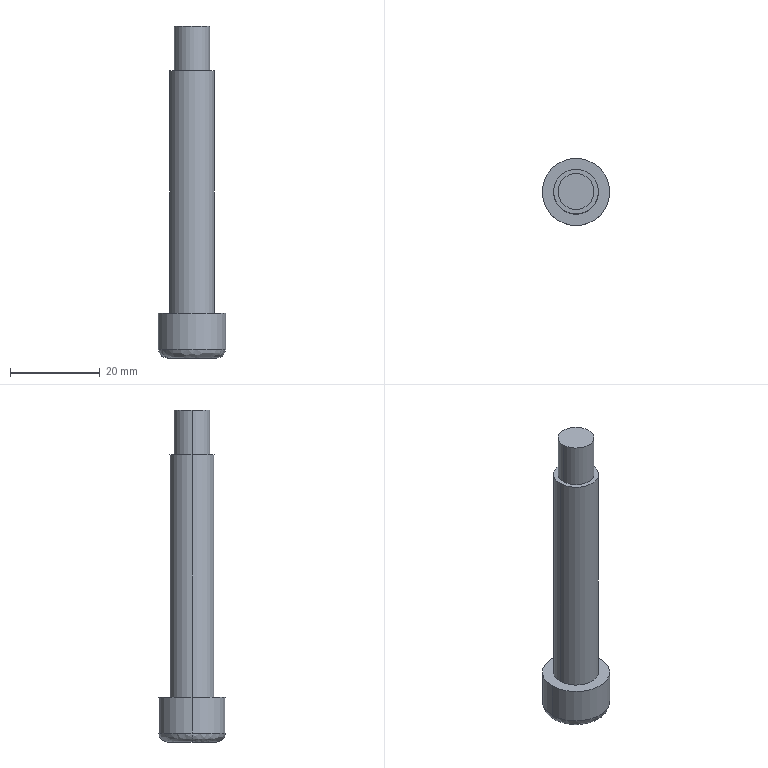Part | STEP file | BULONG BAC M8X10X56 | 1 solid | 19 faces | box 15 x 15 x 74 mm | volume 6196 mm3 | plane 11 | cylinder 6 | spline 2 | commonest cylinder face diameters 8 x2 10 x2 15 x2
STEP:
#1=CARTESIAN_POINT('',(0.,0.,0.));
#2=DIRECTION('',(0.,0.,1.));
#3=DIRECTION('',(1.,0.,0.));
#4=AXIS2_PLACEMENT_3D('',#1,#2,#3);
#5=CARTESIAN_POINT('',(-5.5,0.,0.));
#6=VERTEX_POINT('',#5);
#7=CARTESIAN_POINT('',(5.5,0.,0.));
#8=VERTEX_POINT('',#7);
#9=CARTESIAN_POINT('',(-5.5,0.,0.));
#10=CARTESIAN_POINT('',(-5.5,-11.,0.));
#11=CARTESIAN_POINT('',(5.5,-11.,0.));
#12=CARTESIAN_POINT('',(5.5,0.,0.));
#13=(BOUNDED_CURVE()B_SPLINE_CURVE(3,(#9,#10,#11,#12),.UNSPECIFIED.,.F.,.F.)B_SPLINE_CURVE_WITH_KNOTS((4,4),(0.5,1.),.PIECEWISE_BEZIER_KNOTS.)CURVE()GEOMETRIC_REPRESENTATION_ITEM()RATIONAL_B_SPLINE_CURVE((1.,0.3333,0.3333,1.))REPRESENTATION_ITEM(''));
#14=CARTESIAN_POINT('',(5.5,0.,0.));
#15=CARTESIAN_POINT('',(5.5,-11.,0.));
#16=CARTESIAN_POINT('',(-5.5,-11.,0.));
#17=CARTESIAN_POINT('',(-5.5,0.,0.));
#18=CARTESIAN_POINT('',(6.672,0.,0.));
#19=CARTESIAN_POINT('',(6.672,-13.343,0.));
#20=CARTESIAN_POINT('',(-6.672,-13.343,0.));
#21=CARTESIAN_POINT('',(-6.672,0.,0.));
#22=CARTESIAN_POINT('',(7.5,0.,0.8284));
#23=CARTESIAN_POINT('',(7.5,-15.,0.8284));
#24=CARTESIAN_POINT('',(-7.5,-15.,0.8284));
#25=CARTESIAN_POINT('',(-7.5,0.,0.8284));
#26=CARTESIAN_POINT('',(7.5,0.,2.));
#27=CARTESIAN_POINT('',(7.5,-15.,2.));
#28=CARTESIAN_POINT('',(-7.5,-15.,2.));
#29=CARTESIAN_POINT('',(-7.5,0.,2.));
#30=(BOUNDED_SURFACE()B_SPLINE_SURFACE(3,3,((#14,#15,#16,#17),(#18,#19,#20,#21),(#22,#23,#24,#25),(#26,#27,#28,#29)),.UNSPECIFIED.,.F.,.F.,.F.)B_SPLINE_SURFACE_WITH_KNOTS((4,4),(4,4),(0.,1.),(0.,1.),.PIECEWISE_BEZIER_KNOTS.)GEOMETRIC_REPRESENTATION_ITEM()RATIONAL_B_SPLINE_SURFACE(((1.,0.3333,0.3333,1.),(0.8047,0.2682,0.2682,0.8047),(0.8047,0.2682,0.2682,0.8047),(1.,0.3333,0.3333,1.)))REPRESENTATION_ITEM('')SURFACE());
#31=CARTESIAN_POINT('',(0.,1.));
#32=CARTESIAN_POINT('',(0.,0.));
#33=B_SPLINE_CURVE_WITH_KNOTS('',1,(#31,#32),.UNSPECIFIED.,.F.,.F.,(2,2),(0.5,1.),.PIECEWISE_BEZIER_KNOTS.);
#34=(GEOMETRIC_REPRESENTATION_CONTEXT(2)PARAMETRIC_REPRESENTATION_CONTEXT()REPRESENTATION_CONTEXT('',''));
#35=DEFINITIONAL_REPRESENTATION('',(#33),#34);
#36=PCURVE('',#30,#35);
#37=CARTESIAN_POINT('',(0.,0.,0.));
#38=DIRECTION('',(0.,0.,-1.));
#39=DIRECTION('',(-1.,0.,0.));
#40=AXIS2_PLACEMENT_3D('',#37,#38,#39);
#41=PLANE('',#40);
#42=CARTESIAN_POINT('',(5.5,0.));
#43=CARTESIAN_POINT('',(5.5,-11.));
#44=CARTESIAN_POINT('',(-5.5,-11.));
#45=CARTESIAN_POINT('',(-5.5,0.));
#46=(BOUNDED_CURVE()B_SPLINE_CURVE(3,(#42,#43,#44,#45),.UNSPECIFIED.,.F.,.F.)B_SPLINE_CURVE_WITH_KNOTS((4,4),(0.5,1.),.PIECEWISE_BEZIER_KNOTS.)CURVE()GEOMETRIC_REPRESENTATION_ITEM()RATIONAL_B_SPLINE_CURVE((1.,0.3333,0.3333,1.))REPRESENTATION_ITEM(''));
#47=(GEOMETRIC_REPRESENTATION_CONTEXT(2)PARAMETRIC_REPRESENTATION_CONTEXT()REPRESENTATION_CONTEXT('',''));
#48=DEFINITIONAL_REPRESENTATION('',(#46),#47);
#49=PCURVE('',#41,#48);
#50=SURFACE_CURVE('',#13,(#36,#49),.PCURVE_S1.);
#51=EDGE_CURVE('',#6,#8,#50,.T.);
#52=ORIENTED_EDGE('',*,*,#51,.T.);
#53=CARTESIAN_POINT('',(7.5,0.,2.));
#54=VERTEX_POINT('',#53);
#55=CARTESIAN_POINT('',(5.5,0.,2.));
#56=DIRECTION('',(0.,-1.,0.));
#57=DIRECTION('',(1.,0.,0.));
#58=AXIS2_PLACEMENT_3D('',#55,#56,#57);
#59=CIRCLE('',#58,2.);
#60=CARTESIAN_POINT('',(0.,0.));
#61=CARTESIAN_POINT('',(0.01683,0.));
#62=CARTESIAN_POINT('',(0.04999,0.));
#63=CARTESIAN_POINT('',(0.09843,0.));
#64=CARTESIAN_POINT('',(0.1457,0.));
#65=CARTESIAN_POINT('',(0.192,0.));
#66=CARTESIAN_POINT('',(0.2375,0.));
#67=CARTESIAN_POINT('',(0.2823,0.));
#68=CARTESIAN_POINT('',(0.3265,0.));
#69=CARTESIAN_POINT('',(0.3703,0.));
#70=CARTESIAN_POINT('',(0.4137,0.));
#71=CARTESIAN_POINT('',(0.4569,0.));
#72=CARTESIAN_POINT('',(0.5,0.));
#73=CARTESIAN_POINT('',(0.5431,0.));
#74=CARTESIAN_POINT('',(0.5863,0.));
#75=CARTESIAN_POINT('',(0.6297,0.));
#76=CARTESIAN_POINT('',(0.6735,0.));
#77=CARTESIAN_POINT('',(0.7177,0.));
#78=CARTESIAN_POINT('',(0.7625,0.));
#79=CARTESIAN_POINT('',(0.808,0.));
#80=CARTESIAN_POINT('',(0.8543,0.));
#81=CARTESIAN_POINT('',(0.9016,0.));
#82=CARTESIAN_POINT('',(0.95,0.));
#83=CARTESIAN_POINT('',(0.9832,0.));
#84=CARTESIAN_POINT('',(1.,0.));
#85=B_SPLINE_CURVE_WITH_KNOTS('',3,(#60,#61,#62,#63,#64,#65,#66,#67,#68,#69,#70,#71,#72,#73,#74,#75,#76,#77,#78,#79,#80,#81,#82,#83,#84),.UNSPECIFIED.,.F.,.F.,(4,1,1,1,1,1,1,1,1,1,1,1,1,1,1,1,1,1,1,1,1,1,4),(4.712,4.784,4.855,4.927,4.998,5.069,5.141,5.212,5.284,5.355,5.426,5.498,5.569,5.641,5.712,5.783,5.855,5.926,5.998,6.069,6.14,6.212,6.283),.QUASI_UNIFORM_KNOTS.);
#86=(GEOMETRIC_REPRESENTATION_CONTEXT(2)PARAMETRIC_REPRESENTATION_CONTEXT()REPRESENTATION_CONTEXT('',''));
#87=DEFINITIONAL_REPRESENTATION('',(#85),#86);
#88=PCURVE('',#30,#87);
#89=CARTESIAN_POINT('',(-5.5,0.,0.));
#90=CARTESIAN_POINT('',(-5.5,11.,0.));
#91=CARTESIAN_POINT('',(5.5,11.,0.));
#92=CARTESIAN_POINT('',(5.5,0.,0.));
#93=CARTESIAN_POINT('',(-6.672,0.,0.));
#94=CARTESIAN_POINT('',(-6.672,13.343,0.));
#95=CARTESIAN_POINT('',(6.672,13.343,0.));
#96=CARTESIAN_POINT('',(6.672,0.,0.));
#97=CARTESIAN_POINT('',(-7.5,0.,0.8284));
#98=CARTESIAN_POINT('',(-7.5,15.,0.8284));
#99=CARTESIAN_POINT('',(7.5,15.,0.8284));
#100=CARTESIAN_POINT('',(7.5,0.,0.8284));
#101=CARTESIAN_POINT('',(-7.5,0.,2.));
#102=CARTESIAN_POINT('',(-7.5,15.,2.));
#103=CARTESIAN_POINT('',(7.5,15.,2.));
#104=CARTESIAN_POINT('',(7.5,0.,2.));
#105=(BOUNDED_SURFACE()B_SPLINE_SURFACE(3,3,((#89,#90,#91,#92),(#93,#94,#95,#96),(#97,#98,#99,#100),(#101,#102,#103,#104)),.UNSPECIFIED.,.F.,.F.,.F.)B_SPLINE_SURFACE_WITH_KNOTS((4,4),(4,4),(0.,1.),(0.,1.),.PIECEWISE_BEZIER_KNOTS.)GEOMETRIC_REPRESENTATION_ITEM()RATIONAL_B_SPLINE_SURFACE(((1.,0.3333,0.3333,1.),(0.8047,0.2682,0.2682,0.8047),(0.8047,0.2682,0.2682,0.8047),(1.,0.3333,0.3333,1.)))REPRESENTATION_ITEM('')SURFACE());
#106=CARTESIAN_POINT('',(0.,1.));
#107=CARTESIAN_POINT('',(0.01683,1.));
#108=CARTESIAN_POINT('',(0.04999,1.));
#109=CARTESIAN_POINT('',(0.09843,1.));
#110=CARTESIAN_POINT('',(0.1457,1.));
#111=CARTESIAN_POINT('',(0.192,1.));
#112=CARTESIAN_POINT('',(0.2375,1.));
#113=CARTESIAN_POINT('',(0.2823,1.));
#114=CARTESIAN_POINT('',(0.3265,1.));
#115=CARTESIAN_POINT('',(0.3703,1.));
#116=CARTESIAN_POINT('',(0.4137,1.));
#117=CARTESIAN_POINT('',(0.4569,1.));
#118=CARTESIAN_POINT('',(0.5,1.));
#119=CARTESIAN_POINT('',(0.5431,1.));
#120=CARTESIAN_POINT('',(0.5863,1.));
#121=CARTESIAN_POINT('',(0.6297,1.));
#122=CARTESIAN_POINT('',(0.6735,1.));
#123=CARTESIAN_POINT('',(0.7177,1.));
#124=CARTESIAN_POINT('',(0.7625,1.));
#125=CARTESIAN_POINT('',(0.808,1.));
#126=CARTESIAN_POINT('',(0.8543,1.));
#127=CARTESIAN_POINT('',(0.9016,1.));
#128=CARTESIAN_POINT('',(0.95,1.));
#129=CARTESIAN_POINT('',(0.9832,1.));
#130=CARTESIAN_POINT('',(1.,1.));
#131=B_SPLINE_CURVE_WITH_KNOTS('',3,(#106,#107,#108,#109,#110,#111,#112,#113,#114,#115,#116,#117,#118,#119,#120,#121,#122,#123,#124,#125,#126,#127,#128,#129,#130),.UNSPECIFIED.,.F.,.F.,(4,1,1,1,1,1,1,1,1,1,1,1,1,1,1,1,1,1,1,1,1,1,4),(4.712,4.784,4.855,4.927,4.998,5.069,5.141,5.212,5.284,5.355,5.426,5.498,5.569,5.641,5.712,5.783,5.855,5.926,5.998,6.069,6.14,6.212,6.283),.QUASI_UNIFORM_KNOTS.);
#132=(GEOMETRIC_REPRESENTATION_CONTEXT(2)PARAMETRIC_REPRESENTATION_CONTEXT()REPRESENTATION_CONTEXT('',''));
#133=DEFINITIONAL_REPRESENTATION('',(#131),#132);
#134=PCURVE('',#105,#133);
#135=SURFACE_CURVE('',#59,(#88,#134),.PCURVE_S1.);
#136=EDGE_CURVE('',#8,#54,#135,.T.);
#137=ORIENTED_EDGE('',*,*,#136,.T.);
#138=CARTESIAN_POINT('',(-7.5,0.,2.));
#139=VERTEX_POINT('',#138);
#140=CARTESIAN_POINT('',(0.,0.,2.));
#141=DIRECTION('',(0.,0.,1.));
#142=DIRECTION('',(1.,0.,0.));
#143=AXIS2_PLACEMENT_3D('',#140,#141,#142);
#144=CIRCLE('',#143,7.5);
#145=CARTESIAN_POINT('',(1.,1.));
#146=CARTESIAN_POINT('',(1.,0.9763));
#147=CARTESIAN_POINT('',(1.,0.9319));
#148=CARTESIAN_POINT('',(1.,0.8733));
#149=CARTESIAN_POINT('',(1.,0.8206));
#150=CARTESIAN_POINT('',(1.,0.7724));
#151=CARTESIAN_POINT('',(1.,0.7279));
#152=CARTESIAN_POINT('',(1.,0.6861));
#153=CARTESIAN_POINT('',(1.,0.6465));
#154=CARTESIAN_POINT('',(1.,0.6086));
#155=CARTESIAN_POINT('',(1.,0.5718));
#156=CARTESIAN_POINT('',(1.,0.5357));
#157=CARTESIAN_POINT('',(1.,0.5));
#158=CARTESIAN_POINT('',(1.,0.4643));
#159=CARTESIAN_POINT('',(1.,0.4282));
#160=CARTESIAN_POINT('',(1.,0.3914));
#161=CARTESIAN_POINT('',(1.,0.3535));
#162=CARTESIAN_POINT('',(1.,0.3139));
#163=CARTESIAN_POINT('',(1.,0.2721));
#164=CARTESIAN_POINT('',(1.,0.2276));
#165=CARTESIAN_POINT('',(1.,0.1794));
#166=CARTESIAN_POINT('',(1.,0.1267));
#167=CARTESIAN_POINT('',(1.,0.06805));
#168=CARTESIAN_POINT('',(1.,0.02375));
#169=CARTESIAN_POINT('',(1.,0.));
#170=B_SPLINE_CURVE_WITH_KNOTS('',3,(#145,#146,#147,#148,#149,#150,#151,#152,#153,#154,#155,#156,#157,#158,#159,#160,#161,#162,#163,#164,#165,#166,#167,#168,#169),.UNSPECIFIED.,.F.,.F.,(4,1,1,1,1,1,1,1,1,1,1,1,1,1,1,1,1,1,1,1,1,1,4),(3.142,3.284,3.427,3.57,3.713,3.856,3.998,4.141,4.284,4.427,4.57,4.712,4.855,4.998,5.141,5.284,5.426,5.569,5.712,5.855,5.998,6.14,6.283),.QUASI_UNIFORM_KNOTS.);
#171=(GEOMETRIC_REPRESENTATION_CONTEXT(2)PARAMETRIC_REPRESENTATION_CONTEXT()REPRESENTATION_CONTEXT('',''));
#172=DEFINITIONAL_REPRESENTATION('',(#170),#171);
#173=PCURVE('',#30,#172);
#174=CARTESIAN_POINT('',(0.,0.,0.));
#175=DIRECTION('',(0.,0.,1.));
#176=DIRECTION('',(1.,0.,0.));
#177=AXIS2_PLACEMENT_3D('',#174,#175,#176);
#178=CYLINDRICAL_SURFACE('',#177,7.5);
#179=CARTESIAN_POINT('',(0.,2.));
#180=DIRECTION('',(1.,0.));
#181=VECTOR('',#180,1.);
#182=LINE('',#179,#181);
#183=(GEOMETRIC_REPRESENTATION_CONTEXT(2)PARAMETRIC_REPRESENTATION_CONTEXT()REPRESENTATION_CONTEXT('',''));
#184=DEFINITIONAL_REPRESENTATION('',(#182),#183);
#185=PCURVE('',#178,#184);
#186=SURFACE_CURVE('',#144,(#173,#185),.PCURVE_S1.);
#187=EDGE_CURVE('',#139,#54,#186,.T.);
#188=ORIENTED_EDGE('',*,*,#187,.F.);
#189=CARTESIAN_POINT('',(-5.5,0.,2.));
#190=DIRECTION('',(0.,1.,0.));
#191=DIRECTION('',(-1.,0.,0.));
#192=AXIS2_PLACEMENT_3D('',#189,#190,#191);
#193=CIRCLE('',#192,2.);
#194=CARTESIAN_POINT('',(0.,1.));
#195=CARTESIAN_POINT('',(0.01683,1.));
#196=CARTESIAN_POINT('',(0.04999,1.));
#197=CARTESIAN_POINT('',(0.09843,1.));
#198=CARTESIAN_POINT('',(0.1457,1.));
#199=CARTESIAN_POINT('',(0.192,1.));
#200=CARTESIAN_POINT('',(0.2375,1.));
#201=CARTESIAN_POINT('',(0.2823,1.));
#202=CARTESIAN_POINT('',(0.3265,1.));
#203=CARTESIAN_POINT('',(0.3703,1.));
#204=CARTESIAN_POINT('',(0.4137,1.));
#205=CARTESIAN_POINT('',(0.4569,1.));
#206=CARTESIAN_POINT('',(0.5,1.));
#207=CARTESIAN_POINT('',(0.5431,1.));
#208=CARTESIAN_POINT('',(0.5863,1.));
#209=CARTESIAN_POINT('',(0.6297,1.));
#210=CARTESIAN_POINT('',(0.6735,1.));
#211=CARTESIAN_POINT('',(0.7177,1.));
#212=CARTESIAN_POINT('',(0.7625,1.));
#213=CARTESIAN_POINT('',(0.808,1.));
#214=CARTESIAN_POINT('',(0.8543,1.));
#215=CARTESIAN_POINT('',(0.9016,1.));
#216=CARTESIAN_POINT('',(0.95,1.));
#217=CARTESIAN_POINT('',(0.9832,1.));
#218=CARTESIAN_POINT('',(1.,1.));
#219=B_SPLINE_CURVE_WITH_KNOTS('',3,(#194,#195,#196,#197,#198,#199,#200,#201,#202,#203,#204,#205,#206,#207,#208,#209,#210,#211,#212,#213,#214,#215,#216,#217,#218),.UNSPECIFIED.,.F.,.F.,(4,1,1,1,1,1,1,1,1,1,1,1,1,1,1,1,1,1,1,1,1,1,4),(4.712,4.784,4.855,4.927,4.998,5.069,5.141,5.212,5.284,5.355,5.426,5.498,5.569,5.641,5.712,5.783,5.855,5.926,5.998,6.069,6.14,6.212,6.283),.QUASI_UNIFORM_KNOTS.);
#220=(GEOMETRIC_REPRESENTATION_CONTEXT(2)PARAMETRIC_REPRESENTATION_CONTEXT()REPRESENTATION_CONTEXT('',''));
#221=DEFINITIONAL_REPRESENTATION('',(#219),#220);
#222=PCURVE('',#30,#221);
#223=CARTESIAN_POINT('',(0.,0.));
#224=CARTESIAN_POINT('',(0.01683,0.));
#225=CARTESIAN_POINT('',(0.04999,0.));
#226=CARTESIAN_POINT('',(0.09843,0.));
#227=CARTESIAN_POINT('',(0.1457,0.));
#228=CARTESIAN_POINT('',(0.192,0.));
#229=CARTESIAN_POINT('',(0.2375,0.));
#230=CARTESIAN_POINT('',(0.2823,0.));
#231=CARTESIAN_POINT('',(0.3265,0.));
#232=CARTESIAN_POINT('',(0.3703,0.));
#233=CARTESIAN_POINT('',(0.4137,0.));
#234=CARTESIAN_POINT('',(0.4569,0.));
#235=CARTESIAN_POINT('',(0.5,0.));
#236=CARTESIAN_POINT('',(0.5431,0.));
#237=CARTESIAN_POINT('',(0.5863,0.));
#238=CARTESIAN_POINT('',(0.6297,0.));
#239=CARTESIAN_POINT('',(0.6735,0.));
#240=CARTESIAN_POINT('',(0.7177,0.));
#241=CARTESIAN_POINT('',(0.7625,0.));
#242=CARTESIAN_POINT('',(0.808,0.));
#243=CARTESIAN_POINT('',(0.8543,0.));
#244=CARTESIAN_POINT('',(0.9016,0.));
#245=CARTESIAN_POINT('',(0.95,0.));
#246=CARTESIAN_POINT('',(0.9832,0.));
#247=CARTESIAN_POINT('',(1.,0.));
#248=B_SPLINE_CURVE_WITH_KNOTS('',3,(#223,#224,#225,#226,#227,#228,#229,#230,#231,#232,#233,#234,#235,#236,#237,#238,#239,#240,#241,#242,#243,#244,#245,#246,#247),.UNSPECIFIED.,.F.,.F.,(4,1,1,1,1,1,1,1,1,1,1,1,1,1,1,1,1,1,1,1,1,1,4),(4.712,4.784,4.855,4.927,4.998,5.069,5.141,5.212,5.284,5.355,5.426,5.498,5.569,5.641,5.712,5.783,5.855,5.926,5.998,6.069,6.14,6.212,6.283),.QUASI_UNIFORM_KNOTS.);
#249=(GEOMETRIC_REPRESENTATION_CONTEXT(2)PARAMETRIC_REPRESENTATION_CONTEXT()REPRESENTATION_CONTEXT('',''));
#250=DEFINITIONAL_REPRESENTATION('',(#248),#249);
#251=PCURVE('',#105,#250);
#252=SURFACE_CURVE('',#193,(#222,#251),.PCURVE_S1.);
#253=EDGE_CURVE('',#6,#139,#252,.T.);
#254=ORIENTED_EDGE('',*,*,#253,.F.);
#255=EDGE_LOOP('',(#52,#137,#188,#254));
#256=FACE_BOUND('',#255,.T.);
#257=ADVANCED_FACE('',(#256),#30,.T.);
#258=CARTESIAN_POINT('',(5.,0.,10.));
#259=VERTEX_POINT('',#258);
#260=CARTESIAN_POINT('',(-5.,0.,10.));
#261=VERTEX_POINT('',#260);
#262=CARTESIAN_POINT('',(0.,0.,10.));
#263=DIRECTION('',(0.,0.,1.));
#264=DIRECTION('',(1.,0.,0.));
#265=AXIS2_PLACEMENT_3D('',#262,#263,#264);
#266=CIRCLE('',#265,5.);
#267=CARTESIAN_POINT('',(0.,0.,10.));
#268=DIRECTION('',(0.,0.,1.));
#269=DIRECTION('',(1.,0.,0.));
#270=AXIS2_PLACEMENT_3D('',#267,#268,#269);
#271=CYLINDRICAL_SURFACE('',#270,5.);
#272=CARTESIAN_POINT('',(0.,0.));
#273=DIRECTION('',(1.,0.));
#274=VECTOR('',#273,1.);
#275=LINE('',#272,#274);
#276=(GEOMETRIC_REPRESENTATION_CONTEXT(2)PARAMETRIC_REPRESENTATION_CONTEXT()REPRESENTATION_CONTEXT('',''));
#277=DEFINITIONAL_REPRESENTATION('',(#275),#276);
#278=PCURVE('',#271,#277);
#279=CARTESIAN_POINT('',(0.,0.,10.));
#280=DIRECTION('',(0.,0.,-1.));
#281=DIRECTION('',(-1.,0.,0.));
#282=AXIS2_PLACEMENT_3D('',#279,#280,#281);
#283=PLANE('',#282);
#284=CARTESIAN_POINT('',(-5.,0.));
#285=CARTESIAN_POINT('',(-5.,8.66));
#286=CARTESIAN_POINT('',(2.5,4.33));
#287=CARTESIAN_POINT('',(10.,0.));
#288=CARTESIAN_POINT('',(2.5,-4.33));
#289=CARTESIAN_POINT('',(-5.,-8.66));
#290=CARTESIAN_POINT('',(-5.,0.));
#291=(BOUNDED_CURVE()B_SPLINE_CURVE(2,(#284,#285,#286,#287,#288,#289,#290),.UNSPECIFIED.,.T.,.F.)B_SPLINE_CURVE_WITH_KNOTS((1,2,2,2,2,1),(-2.094,0.,2.094,4.189,6.283,8.378),.UNSPECIFIED.)CURVE()GEOMETRIC_REPRESENTATION_ITEM()RATIONAL_B_SPLINE_CURVE((1.,0.5,1.,0.5,1.,0.5,1.))REPRESENTATION_ITEM(''));
#292=(GEOMETRIC_REPRESENTATION_CONTEXT(2)PARAMETRIC_REPRESENTATION_CONTEXT()REPRESENTATION_CONTEXT('',''));
#293=DEFINITIONAL_REPRESENTATION('',(#291),#292);
#294=PCURVE('',#283,#293);
#295=SURFACE_CURVE('',#266,(#278,#294),.PCURVE_S1.);
#296=EDGE_CURVE('',#259,#261,#295,.T.);
#297=ORIENTED_EDGE('',*,*,#296,.T.);
#298=CARTESIAN_POINT('',(-5.,0.,64.));
#299=VERTEX_POINT('',#298);
#300=CARTESIAN_POINT('',(-5.,0.,10.));
#301=DIRECTION('',(0.,0.,1.));
#302=VECTOR('',#301,1.);
#303=LINE('',#300,#302);
#304=CARTESIAN_POINT('',(3.142,0.));
#305=DIRECTION('',(0.,1.));
#306=VECTOR('',#305,1.);
#307=LINE('',#304,#306);
#308=(GEOMETRIC_REPRESENTATION_CONTEXT(2)PARAMETRIC_REPRESENTATION_CONTEXT()REPRESENTATION_CONTEXT('',''));
#309=DEFINITIONAL_REPRESENTATION('',(#307),#308);
#310=PCURVE('',#271,#309);
#311=CARTESIAN_POINT('',(0.,0.,10.));
#312=DIRECTION('',(0.,0.,1.));
#313=DIRECTION('',(1.,0.,0.));
#314=AXIS2_PLACEMENT_3D('',#311,#312,#313);
#315=CYLINDRICAL_SURFACE('',#314,5.);
#316=CARTESIAN_POINT('',(3.142,0.));
#317=DIRECTION('',(0.,1.));
#318=VECTOR('',#317,1.);
#319=LINE('',#316,#318);
#320=(GEOMETRIC_REPRESENTATION_CONTEXT(2)PARAMETRIC_REPRESENTATION_CONTEXT()REPRESENTATION_CONTEXT('',''));
#321=DEFINITIONAL_REPRESENTATION('',(#319),#320);
#322=PCURVE('',#315,#321);
#323=SURFACE_CURVE('',#303,(#310,#322),.PCURVE_S1.);
#324=EDGE_CURVE('',#261,#299,#323,.T.);
#325=ORIENTED_EDGE('',*,*,#324,.T.);
#326=CARTESIAN_POINT('',(5.,0.,64.));
#327=VERTEX_POINT('',#326);
#328=CARTESIAN_POINT('',(0.,0.,64.));
#329=DIRECTION('',(0.,0.,-1.));
#330=DIRECTION('',(1.,0.,0.));
#331=AXIS2_PLACEMENT_3D('',#328,#329,#330);
#332=CIRCLE('',#331,5.);
#333=CARTESIAN_POINT('',(6.283,54.));
#334=DIRECTION('',(-1.,0.));
#335=VECTOR('',#334,1.);
#336=LINE('',#333,#335);
#337=(GEOMETRIC_REPRESENTATION_CONTEXT(2)PARAMETRIC_REPRESENTATION_CONTEXT()REPRESENTATION_CONTEXT('',''));
#338=DEFINITIONAL_REPRESENTATION('',(#336),#337);
#339=PCURVE('',#271,#338);
#340=CARTESIAN_POINT('',(0.,0.,64.));
#341=DIRECTION('',(0.,0.,-1.));
#342=DIRECTION('',(-1.,0.,0.));
#343=AXIS2_PLACEMENT_3D('',#340,#341,#342);
#344=PLANE('',#343);
#345=CARTESIAN_POINT('',(0.,0.));
#346=DIRECTION('',(-1.,0.));
#347=AXIS2_PLACEMENT_2D('',#345,#346);
#348=CIRCLE('',#347,5.);
#349=(GEOMETRIC_REPRESENTATION_CONTEXT(2)PARAMETRIC_REPRESENTATION_CONTEXT()REPRESENTATION_CONTEXT('',''));
#350=DEFINITIONAL_REPRESENTATION('',(#348),#349);
#351=PCURVE('',#344,#350);
#352=SURFACE_CURVE('',#332,(#339,#351),.PCURVE_S1.);
#353=EDGE_CURVE('',#299,#327,#352,.T.);
#354=ORIENTED_EDGE('',*,*,#353,.T.);
#355=CARTESIAN_POINT('',(5.,0.,10.));
#356=DIRECTION('',(0.,0.,1.));
#357=VECTOR('',#356,1.);
#358=LINE('',#355,#357);
#359=CARTESIAN_POINT('',(0.,0.));
#360=DIRECTION('',(0.,1.));
#361=VECTOR('',#360,1.);
#362=LINE('',#359,#361);
#363=(GEOMETRIC_REPRESENTATION_CONTEXT(2)PARAMETRIC_REPRESENTATION_CONTEXT()REPRESENTATION_CONTEXT('',''));
#364=DEFINITIONAL_REPRESENTATION('',(#362),#363);
#365=PCURVE('',#271,#364);
#366=CARTESIAN_POINT('',(6.283,0.));
#367=DIRECTION('',(0.,1.));
#368=VECTOR('',#367,1.);
#369=LINE('',#366,#368);
#370=(GEOMETRIC_REPRESENTATION_CONTEXT(2)PARAMETRIC_REPRESENTATION_CONTEXT()REPRESENTATION_CONTEXT('',''));
#371=DEFINITIONAL_REPRESENTATION('',(#369),#370);
#372=PCURVE('',#315,#371);
#373=SURFACE_CURVE('',#358,(#365,#372),.PCURVE_S1.);
#374=EDGE_CURVE('',#259,#327,#373,.T.);
#375=ORIENTED_EDGE('',*,*,#374,.F.);
#376=EDGE_LOOP('',(#297,#325,#354,#375));
#377=FACE_BOUND('',#376,.T.);
#378=ADVANCED_FACE('',(#377),#271,.T.);
#379=CARTESIAN_POINT('',(0.,0.,2.));
#380=DIRECTION('',(0.,0.,1.));
#381=DIRECTION('',(1.,0.,0.));
#382=AXIS2_PLACEMENT_3D('',#379,#380,#381);
#383=CIRCLE('',#382,7.5);
#384=CARTESIAN_POINT('',(0.,0.,0.));
#385=DIRECTION('',(0.,0.,1.));
#386=DIRECTION('',(1.,0.,0.));
#387=AXIS2_PLACEMENT_3D('',#384,#385,#386);
#388=CYLINDRICAL_SURFACE('',#387,7.5);
#389=CARTESIAN_POINT('',(0.,2.));
#390=DIRECTION('',(1.,0.));
#391=VECTOR('',#390,1.);
#392=LINE('',#389,#391);
#393=(GEOMETRIC_REPRESENTATION_CONTEXT(2)PARAMETRIC_REPRESENTATION_CONTEXT()REPRESENTATION_CONTEXT('',''));
#394=DEFINITIONAL_REPRESENTATION('',(#392),#393);
#395=PCURVE('',#388,#394);
#396=CARTESIAN_POINT('',(1.,1.));
#397=CARTESIAN_POINT('',(1.,0.9763));
#398=CARTESIAN_POINT('',(1.,0.9319));
#399=CARTESIAN_POINT('',(1.,0.8733));
#400=CARTESIAN_POINT('',(1.,0.8206));
#401=CARTESIAN_POINT('',(1.,0.7724));
#402=CARTESIAN_POINT('',(1.,0.7279));
#403=CARTESIAN_POINT('',(1.,0.6861));
#404=CARTESIAN_POINT('',(1.,0.6465));
#405=CARTESIAN_POINT('',(1.,0.6086));
#406=CARTESIAN_POINT('',(1.,0.5718));
#407=CARTESIAN_POINT('',(1.,0.5357));
#408=CARTESIAN_POINT('',(1.,0.5));
#409=CARTESIAN_POINT('',(1.,0.4643));
#410=CARTESIAN_POINT('',(1.,0.4282));
#411=CARTESIAN_POINT('',(1.,0.3914));
#412=CARTESIAN_POINT('',(1.,0.3535));
#413=CARTESIAN_POINT('',(1.,0.3139));
#414=CARTESIAN_POINT('',(1.,0.2721));
#415=CARTESIAN_POINT('',(1.,0.2276));
#416=CARTESIAN_POINT('',(1.,0.1794));
#417=CARTESIAN_POINT('',(1.,0.1267));
#418=CARTESIAN_POINT('',(1.,0.06805));
#419=CARTESIAN_POINT('',(1.,0.02375));
#420=CARTESIAN_POINT('',(1.,0.));
#421=B_SPLINE_CURVE_WITH_KNOTS('',3,(#396,#397,#398,#399,#400,#401,#402,#403,#404,#405,#406,#407,#408,#409,#410,#411,#412,#413,#414,#415,#416,#417,#418,#419,#420),.UNSPECIFIED.,.F.,.F.,(4,1,1,1,1,1,1,1,1,1,1,1,1,1,1,1,1,1,1,1,1,1,4),(0.,0.1428,0.2856,0.4284,0.5712,0.714,0.8568,0.9996,1.142,1.285,1.428,1.571,1.714,1.856,1.999,2.142,2.285,2.428,2.57,2.713,2.856,2.999,3.142),.QUASI_UNIFORM_KNOTS.);
#422=(GEOMETRIC_REPRESENTATION_CONTEXT(2)PARAMETRIC_REPRESENTATION_CONTEXT()REPRESENTATION_CONTEXT('',''));
#423=DEFINITIONAL_REPRESENTATION('',(#421),#422);
#424=PCURVE('',#105,#423);
#425=SURFACE_CURVE('',#383,(#395,#424),.PCURVE_S1.);
#426=EDGE_CURVE('',#54,#139,#425,.T.);
#427=ORIENTED_EDGE('',*,*,#426,.T.);
#428=CARTESIAN_POINT('',(-7.5,0.,10.));
#429=VERTEX_POINT('',#428);
#430=CARTESIAN_POINT('',(-7.5,0.,0.));
#431=DIRECTION('',(0.,0.,1.));
#432=VECTOR('',#431,1.);
#433=LINE('',#430,#432);
#434=CARTESIAN_POINT('',(3.142,0.));
#435=DIRECTION('',(0.,1.));
#436=VECTOR('',#435,1.);
#437=LINE('',#434,#436);
#438=(GEOMETRIC_REPRESENTATION_CONTEXT(2)PARAMETRIC_REPRESENTATION_CONTEXT()REPRESENTATION_CONTEXT('',''));
#439=DEFINITIONAL_REPRESENTATION('',(#437),#438);
#440=PCURVE('',#388,#439);
#441=CARTESIAN_POINT('',(3.142,0.));
#442=DIRECTION('',(0.,1.));
#443=VECTOR('',#442,1.);
#444=LINE('',#441,#443);
#445=(GEOMETRIC_REPRESENTATION_CONTEXT(2)PARAMETRIC_REPRESENTATION_CONTEXT()REPRESENTATION_CONTEXT('',''));
#446=DEFINITIONAL_REPRESENTATION('',(#444),#445);
#447=PCURVE('',#178,#446);
#448=SURFACE_CURVE('',#433,(#440,#447),.PCURVE_S1.);
#449=EDGE_CURVE('',#139,#429,#448,.T.);
#450=ORIENTED_EDGE('',*,*,#449,.T.);
#451=CARTESIAN_POINT('',(7.5,0.,10.));
#452=VERTEX_POINT('',#451);
#453=CARTESIAN_POINT('',(0.,0.,10.));
#454=DIRECTION('',(0.,0.,-1.));
#455=DIRECTION('',(1.,0.,0.));
#456=AXIS2_PLACEMENT_3D('',#453,#454,#455);
#457=CIRCLE('',#456,7.5);
#458=CARTESIAN_POINT('',(6.283,10.));
#459=DIRECTION('',(-1.,0.));
#460=VECTOR('',#459,1.);
#461=LINE('',#458,#460);
#462=(GEOMETRIC_REPRESENTATION_CONTEXT(2)PARAMETRIC_REPRESENTATION_CONTEXT()REPRESENTATION_CONTEXT('',''));
#463=DEFINITIONAL_REPRESENTATION('',(#461),#462);
#464=PCURVE('',#388,#463);
#465=CARTESIAN_POINT('',(0.,0.));
#466=DIRECTION('',(-1.,0.));
#467=AXIS2_PLACEMENT_2D('',#465,#466);
#468=CIRCLE('',#467,7.5);
#469=(GEOMETRIC_REPRESENTATION_CONTEXT(2)PARAMETRIC_REPRESENTATION_CONTEXT()REPRESENTATION_CONTEXT('',''));
#470=DEFINITIONAL_REPRESENTATION('',(#468),#469);
#471=PCURVE('',#283,#470);
#472=SURFACE_CURVE('',#457,(#464,#471),.PCURVE_S1.);
#473=EDGE_CURVE('',#429,#452,#472,.T.);
#474=ORIENTED_EDGE('',*,*,#473,.T.);
#475=CARTESIAN_POINT('',(7.5,0.,0.));
#476=DIRECTION('',(0.,0.,1.));
#477=VECTOR('',#476,1.);
#478=LINE('',#475,#477);
#479=CARTESIAN_POINT('',(0.,0.));
#480=DIRECTION('',(0.,1.));
#481=VECTOR('',#480,1.);
#482=LINE('',#479,#481);
#483=(GEOMETRIC_REPRESENTATION_CONTEXT(2)PARAMETRIC_REPRESENTATION_CONTEXT()REPRESENTATION_CONTEXT('',''));
#484=DEFINITIONAL_REPRESENTATION('',(#482),#483);
#485=PCURVE('',#388,#484);
#486=CARTESIAN_POINT('',(6.283,0.));
#487=DIRECTION('',(0.,1.));
#488=VECTOR('',#487,1.);
#489=LINE('',#486,#488);
#490=(GEOMETRIC_REPRESENTATION_CONTEXT(2)PARAMETRIC_REPRESENTATION_CONTEXT()REPRESENTATION_CONTEXT('',''));
#491=DEFINITIONAL_REPRESENTATION('',(#489),#490);
#492=PCURVE('',#178,#491);
#493=SURFACE_CURVE('',#478,(#485,#492),.PCURVE_S1.);
#494=EDGE_CURVE('',#54,#452,#493,.T.);
#495=ORIENTED_EDGE('',*,*,#494,.F.);
#496=EDGE_LOOP('',(#427,#450,#474,#495));
#497=FACE_BOUND('',#496,.T.);
#498=ADVANCED_FACE('',(#497),#388,.T.);
#499=CARTESIAN_POINT('',(4.,0.,64.));
#500=VERTEX_POINT('',#499);
#501=CARTESIAN_POINT('',(-4.,0.,64.));
#502=VERTEX_POINT('',#501);
#503=CARTESIAN_POINT('',(0.,0.,64.));
#504=DIRECTION('',(0.,0.,1.));
#505=DIRECTION('',(1.,0.,0.));
#506=AXIS2_PLACEMENT_3D('',#503,#504,#505);
#507=CIRCLE('',#506,4.);
#508=CARTESIAN_POINT('',(0.,0.,64.));
#509=DIRECTION('',(0.,0.,1.));
#510=DIRECTION('',(1.,0.,0.));
#511=AXIS2_PLACEMENT_3D('',#508,#509,#510);
#512=CYLINDRICAL_SURFACE('',#511,4.);
#513=CARTESIAN_POINT('',(0.,0.));
#514=DIRECTION('',(1.,0.));
#515=VECTOR('',#514,1.);
#516=LINE('',#513,#515);
#517=(GEOMETRIC_REPRESENTATION_CONTEXT(2)PARAMETRIC_REPRESENTATION_CONTEXT()REPRESENTATION_CONTEXT('',''));
#518=DEFINITIONAL_REPRESENTATION('',(#516),#517);
#519=PCURVE('',#512,#518);
#520=CARTESIAN_POINT('',(-4.,0.));
#521=CARTESIAN_POINT('',(-4.,6.928));
#522=CARTESIAN_POINT('',(2.,3.464));
#523=CARTESIAN_POINT('',(8.,0.));
#524=CARTESIAN_POINT('',(2.,-3.464));
#525=CARTESIAN_POINT('',(-4.,-6.928));
#526=CARTESIAN_POINT('',(-4.,0.));
#527=(BOUNDED_CURVE()B_SPLINE_CURVE(2,(#520,#521,#522,#523,#524,#525,#526),.UNSPECIFIED.,.T.,.F.)B_SPLINE_CURVE_WITH_KNOTS((1,2,2,2,2,1),(-2.094,0.,2.094,4.189,6.283,8.378),.UNSPECIFIED.)CURVE()GEOMETRIC_REPRESENTATION_ITEM()RATIONAL_B_SPLINE_CURVE((1.,0.5,1.,0.5,1.,0.5,1.))REPRESENTATION_ITEM(''));
#528=(GEOMETRIC_REPRESENTATION_CONTEXT(2)PARAMETRIC_REPRESENTATION_CONTEXT()REPRESENTATION_CONTEXT('',''));
#529=DEFINITIONAL_REPRESENTATION('',(#527),#528);
#530=PCURVE('',#344,#529);
#531=SURFACE_CURVE('',#507,(#519,#530),.PCURVE_S1.);
#532=EDGE_CURVE('',#500,#502,#531,.T.);
#533=ORIENTED_EDGE('',*,*,#532,.T.);
#534=CARTESIAN_POINT('',(-4.,0.,74.));
#535=VERTEX_POINT('',#534);
#536=CARTESIAN_POINT('',(-4.,0.,64.));
#537=DIRECTION('',(0.,0.,1.));
#538=VECTOR('',#537,1.);
#539=LINE('',#536,#538);
#540=CARTESIAN_POINT('',(3.142,0.));
#541=DIRECTION('',(0.,1.));
#542=VECTOR('',#541,1.);
#543=LINE('',#540,#542);
#544=(GEOMETRIC_REPRESENTATION_CONTEXT(2)PARAMETRIC_REPRESENTATION_CONTEXT()REPRESENTATION_CONTEXT('',''));
#545=DEFINITIONAL_REPRESENTATION('',(#543),#544);
#546=PCURVE('',#512,#545);
#547=CARTESIAN_POINT('',(0.,0.,64.));
#548=DIRECTION('',(0.,0.,1.));
#549=DIRECTION('',(1.,0.,0.));
#550=AXIS2_PLACEMENT_3D('',#547,#548,#549);
#551=CYLINDRICAL_SURFACE('',#550,4.);
#552=CARTESIAN_POINT('',(3.142,0.));
#553=DIRECTION('',(0.,1.));
#554=VECTOR('',#553,1.);
#555=LINE('',#552,#554);
#556=(GEOMETRIC_REPRESENTATION_CONTEXT(2)PARAMETRIC_REPRESENTATION_CONTEXT()REPRESENTATION_CONTEXT('',''));
#557=DEFINITIONAL_REPRESENTATION('',(#555),#556);
#558=PCURVE('',#551,#557);
#559=SURFACE_CURVE('',#539,(#546,#558),.PCURVE_S1.);
#560=EDGE_CURVE('',#502,#535,#559,.T.);
#561=ORIENTED_EDGE('',*,*,#560,.T.);
#562=CARTESIAN_POINT('',(4.,0.,74.));
#563=VERTEX_POINT('',#562);
#564=CARTESIAN_POINT('',(0.,0.,74.));
#565=DIRECTION('',(0.,0.,-1.));
#566=DIRECTION('',(1.,0.,0.));
#567=AXIS2_PLACEMENT_3D('',#564,#565,#566);
#568=CIRCLE('',#567,4.);
#569=CARTESIAN_POINT('',(6.283,10.));
#570=DIRECTION('',(-1.,0.));
#571=VECTOR('',#570,1.);
#572=LINE('',#569,#571);
#573=(GEOMETRIC_REPRESENTATION_CONTEXT(2)PARAMETRIC_REPRESENTATION_CONTEXT()REPRESENTATION_CONTEXT('',''));
#574=DEFINITIONAL_REPRESENTATION('',(#572),#573);
#575=PCURVE('',#512,#574);
#576=CARTESIAN_POINT('',(0.,0.,74.));
#577=DIRECTION('',(0.,0.,-1.));
#578=DIRECTION('',(-1.,0.,0.));
#579=AXIS2_PLACEMENT_3D('',#576,#577,#578);
#580=PLANE('',#579);
#581=CARTESIAN_POINT('',(0.,0.));
#582=DIRECTION('',(-1.,0.));
#583=AXIS2_PLACEMENT_2D('',#581,#582);
#584=CIRCLE('',#583,4.);
#585=(GEOMETRIC_REPRESENTATION_CONTEXT(2)PARAMETRIC_REPRESENTATION_CONTEXT()REPRESENTATION_CONTEXT('',''));
#586=DEFINITIONAL_REPRESENTATION('',(#584),#585);
#587=PCURVE('',#580,#586);
#588=SURFACE_CURVE('',#568,(#575,#587),.PCURVE_S1.);
#589=EDGE_CURVE('',#535,#563,#588,.T.);
#590=ORIENTED_EDGE('',*,*,#589,.T.);
#591=CARTESIAN_POINT('',(4.,0.,64.));
#592=DIRECTION('',(0.,0.,1.));
#593=VECTOR('',#592,1.);
#594=LINE('',#591,#593);
#595=CARTESIAN_POINT('',(0.,0.));
#596=DIRECTION('',(0.,1.));
#597=VECTOR('',#596,1.);
#598=LINE('',#595,#597);
#599=(GEOMETRIC_REPRESENTATION_CONTEXT(2)PARAMETRIC_REPRESENTATION_CONTEXT()REPRESENTATION_CONTEXT('',''));
#600=DEFINITIONAL_REPRESENTATION('',(#598),#599);
#601=PCURVE('',#512,#600);
#602=CARTESIAN_POINT('',(6.283,0.));
#603=DIRECTION('',(0.,1.));
#604=VECTOR('',#603,1.);
#605=LINE('',#602,#604);
#606=(GEOMETRIC_REPRESENTATION_CONTEXT(2)PARAMETRIC_REPRESENTATION_CONTEXT()REPRESENTATION_CONTEXT('',''));
#607=DEFINITIONAL_REPRESENTATION('',(#605),#606);
#608=PCURVE('',#551,#607);
#609=SURFACE_CURVE('',#594,(#601,#608),.PCURVE_S1.);
#610=EDGE_CURVE('',#500,#563,#609,.T.);
#611=ORIENTED_EDGE('',*,*,#610,.F.);
#612=EDGE_LOOP('',(#533,#561,#590,#611));
#613=FACE_BOUND('',#612,.T.);
#614=ADVANCED_FACE('',(#613),#512,.T.);
#615=ORIENTED_EDGE('',*,*,#324,.F.);
#616=CARTESIAN_POINT('',(0.,0.,10.));
#617=DIRECTION('',(0.,0.,1.));
#618=DIRECTION('',(1.,0.,0.));
#619=AXIS2_PLACEMENT_3D('',#616,#617,#618);
#620=CIRCLE('',#619,5.);
#621=CARTESIAN_POINT('',(0.,0.));
#622=DIRECTION('',(1.,0.));
#623=VECTOR('',#622,1.);
#624=LINE('',#621,#623);
#625=(GEOMETRIC_REPRESENTATION_CONTEXT(2)PARAMETRIC_REPRESENTATION_CONTEXT()REPRESENTATION_CONTEXT('',''));
#626=DEFINITIONAL_REPRESENTATION('',(#624),#625);
#627=PCURVE('',#315,#626);
#628=CARTESIAN_POINT('',(-5.,0.));
#629=CARTESIAN_POINT('',(-5.,8.66));
#630=CARTESIAN_POINT('',(2.5,4.33));
#631=CARTESIAN_POINT('',(10.,0.));
#632=CARTESIAN_POINT('',(2.5,-4.33));
#633=CARTESIAN_POINT('',(-5.,-8.66));
#634=CARTESIAN_POINT('',(-5.,0.));
#635=(BOUNDED_CURVE()B_SPLINE_CURVE(2,(#628,#629,#630,#631,#632,#633,#634),.UNSPECIFIED.,.T.,.F.)B_SPLINE_CURVE_WITH_KNOTS((1,2,2,2,2,1),(-2.094,0.,2.094,4.189,6.283,8.378),.UNSPECIFIED.)CURVE()GEOMETRIC_REPRESENTATION_ITEM()RATIONAL_B_SPLINE_CURVE((1.,0.5,1.,0.5,1.,0.5,1.))REPRESENTATION_ITEM(''));
#636=(GEOMETRIC_REPRESENTATION_CONTEXT(2)PARAMETRIC_REPRESENTATION_CONTEXT()REPRESENTATION_CONTEXT('',''));
#637=DEFINITIONAL_REPRESENTATION('',(#635),#636);
#638=PCURVE('',#283,#637);
#639=SURFACE_CURVE('',#620,(#627,#638),.PCURVE_S1.);
#640=EDGE_CURVE('',#261,#259,#639,.T.);
#641=ORIENTED_EDGE('',*,*,#640,.T.);
#642=ORIENTED_EDGE('',*,*,#374,.T.);
#643=CARTESIAN_POINT('',(0.,0.,64.));
#644=DIRECTION('',(0.,0.,-1.));
#645=DIRECTION('',(1.,0.,0.));
#646=AXIS2_PLACEMENT_3D('',#643,#644,#645);
#647=CIRCLE('',#646,5.);
#648=CARTESIAN_POINT('',(6.283,54.));
#649=DIRECTION('',(-1.,0.));
#650=VECTOR('',#649,1.);
#651=LINE('',#648,#650);
#652=(GEOMETRIC_REPRESENTATION_CONTEXT(2)PARAMETRIC_REPRESENTATION_CONTEXT()REPRESENTATION_CONTEXT('',''));
#653=DEFINITIONAL_REPRESENTATION('',(#651),#652);
#654=PCURVE('',#315,#653);
#655=CARTESIAN_POINT('',(0.,0.));
#656=DIRECTION('',(-1.,0.));
#657=AXIS2_PLACEMENT_2D('',#655,#656);
#658=CIRCLE('',#657,5.);
#659=(GEOMETRIC_REPRESENTATION_CONTEXT(2)PARAMETRIC_REPRESENTATION_CONTEXT()REPRESENTATION_CONTEXT('',''));
#660=DEFINITIONAL_REPRESENTATION('',(#658),#659);
#661=PCURVE('',#344,#660);
#662=SURFACE_CURVE('',#647,(#654,#661),.PCURVE_S1.);
#663=EDGE_CURVE('',#327,#299,#662,.T.);
#664=ORIENTED_EDGE('',*,*,#663,.T.);
#665=EDGE_LOOP('',(#615,#641,#642,#664));
#666=FACE_BOUND('',#665,.T.);
#667=ADVANCED_FACE('',(#666),#315,.T.);
#668=ORIENTED_EDGE('',*,*,#296,.F.);
#669=ORIENTED_EDGE('',*,*,#640,.F.);
#670=EDGE_LOOP('',(#668,#669));
#671=FACE_BOUND('',#670,.T.);
#672=CARTESIAN_POINT('',(0.,0.,10.));
#673=DIRECTION('',(0.,0.,-1.));
#674=DIRECTION('',(1.,0.,0.));
#675=AXIS2_PLACEMENT_3D('',#672,#673,#674);
#676=CIRCLE('',#675,7.5);
#677=CARTESIAN_POINT('',(0.,0.));
#678=DIRECTION('',(-1.,0.));
#679=AXIS2_PLACEMENT_2D('',#677,#678);
#680=CIRCLE('',#679,7.5);
#681=(GEOMETRIC_REPRESENTATION_CONTEXT(2)PARAMETRIC_REPRESENTATION_CONTEXT()REPRESENTATION_CONTEXT('',''));
#682=DEFINITIONAL_REPRESENTATION('',(#680),#681);
#683=PCURVE('',#283,#682);
#684=CARTESIAN_POINT('',(6.283,10.));
#685=DIRECTION('',(-1.,0.));
#686=VECTOR('',#685,1.);
#687=LINE('',#684,#686);
#688=(GEOMETRIC_REPRESENTATION_CONTEXT(2)PARAMETRIC_REPRESENTATION_CONTEXT()REPRESENTATION_CONTEXT('',''));
#689=DEFINITIONAL_REPRESENTATION('',(#687),#688);
#690=PCURVE('',#178,#689);
#691=SURFACE_CURVE('',#676,(#683,#690),.PCURVE_S1.);
#692=EDGE_CURVE('',#452,#429,#691,.T.);
#693=ORIENTED_EDGE('',*,*,#692,.F.);
#694=ORIENTED_EDGE('',*,*,#473,.F.);
#695=EDGE_LOOP('',(#693,#694));
#696=FACE_BOUND('',#695,.T.);
#697=ADVANCED_FACE('',(#671,#696),#283,.F.);
#698=ORIENTED_EDGE('',*,*,#532,.F.);
#699=CARTESIAN_POINT('',(0.,0.,64.));
#700=DIRECTION('',(0.,0.,1.));
#701=DIRECTION('',(1.,0.,0.));
#702=AXIS2_PLACEMENT_3D('',#699,#700,#701);
#703=CIRCLE('',#702,4.);
#704=CARTESIAN_POINT('',(-4.,0.));
#705=CARTESIAN_POINT('',(-4.,6.928));
#706=CARTESIAN_POINT('',(2.,3.464));
#707=CARTESIAN_POINT('',(8.,0.));
#708=CARTESIAN_POINT('',(2.,-3.464));
#709=CARTESIAN_POINT('',(-4.,-6.928));
#710=CARTESIAN_POINT('',(-4.,0.));
#711=(BOUNDED_CURVE()B_SPLINE_CURVE(2,(#704,#705,#706,#707,#708,#709,#710),.UNSPECIFIED.,.T.,.F.)B_SPLINE_CURVE_WITH_KNOTS((1,2,2,2,2,1),(-2.094,0.,2.094,4.189,6.283,8.378),.UNSPECIFIED.)CURVE()GEOMETRIC_REPRESENTATION_ITEM()RATIONAL_B_SPLINE_CURVE((1.,0.5,1.,0.5,1.,0.5,1.))REPRESENTATION_ITEM(''));
#712=(GEOMETRIC_REPRESENTATION_CONTEXT(2)PARAMETRIC_REPRESENTATION_CONTEXT()REPRESENTATION_CONTEXT('',''));
#713=DEFINITIONAL_REPRESENTATION('',(#711),#712);
#714=PCURVE('',#344,#713);
#715=CARTESIAN_POINT('',(0.,0.));
#716=DIRECTION('',(1.,0.));
#717=VECTOR('',#716,1.);
#718=LINE('',#715,#717);
#719=(GEOMETRIC_REPRESENTATION_CONTEXT(2)PARAMETRIC_REPRESENTATION_CONTEXT()REPRESENTATION_CONTEXT('',''));
#720=DEFINITIONAL_REPRESENTATION('',(#718),#719);
#721=PCURVE('',#551,#720);
#722=SURFACE_CURVE('',#703,(#714,#721),.PCURVE_S1.);
#723=EDGE_CURVE('',#502,#500,#722,.T.);
#724=ORIENTED_EDGE('',*,*,#723,.F.);
#725=EDGE_LOOP('',(#698,#724));
#726=FACE_BOUND('',#725,.T.);
#727=ORIENTED_EDGE('',*,*,#663,.F.);
#728=ORIENTED_EDGE('',*,*,#353,.F.);
#729=EDGE_LOOP('',(#727,#728));
#730=FACE_BOUND('',#729,.T.);
#731=ADVANCED_FACE('',(#726,#730),#344,.F.);
#732=ORIENTED_EDGE('',*,*,#449,.F.);
#733=ORIENTED_EDGE('',*,*,#187,.T.);
#734=ORIENTED_EDGE('',*,*,#494,.T.);
#735=ORIENTED_EDGE('',*,*,#692,.T.);
#736=EDGE_LOOP('',(#732,#733,#734,#735));
#737=FACE_BOUND('',#736,.T.);
#738=ADVANCED_FACE('',(#737),#178,.T.);
#739=ORIENTED_EDGE('',*,*,#560,.F.);
#740=ORIENTED_EDGE('',*,*,#723,.T.);
#741=ORIENTED_EDGE('',*,*,#610,.T.);
#742=CARTESIAN_POINT('',(0.,0.,74.));
#743=DIRECTION('',(0.,0.,-1.));
#744=DIRECTION('',(1.,0.,0.));
#745=AXIS2_PLACEMENT_3D('',#742,#743,#744);
#746=CIRCLE('',#745,4.);
#747=CARTESIAN_POINT('',(6.283,10.));
#748=DIRECTION('',(-1.,0.));
#749=VECTOR('',#748,1.);
#750=LINE('',#747,#749);
#751=(GEOMETRIC_REPRESENTATION_CONTEXT(2)PARAMETRIC_REPRESENTATION_CONTEXT()REPRESENTATION_CONTEXT('',''));
#752=DEFINITIONAL_REPRESENTATION('',(#750),#751);
#753=PCURVE('',#551,#752);
#754=CARTESIAN_POINT('',(0.,0.));
#755=DIRECTION('',(-1.,0.));
#756=AXIS2_PLACEMENT_2D('',#754,#755);
#757=CIRCLE('',#756,4.);
#758=(GEOMETRIC_REPRESENTATION_CONTEXT(2)PARAMETRIC_REPRESENTATION_CONTEXT()REPRESENTATION_CONTEXT('',''));
#759=DEFINITIONAL_REPRESENTATION('',(#757),#758);
#760=PCURVE('',#580,#759);
#761=SURFACE_CURVE('',#746,(#753,#760),.PCURVE_S1.);
#762=EDGE_CURVE('',#563,#535,#761,.T.);
#763=ORIENTED_EDGE('',*,*,#762,.T.);
#764=EDGE_LOOP('',(#739,#740,#741,#763));
#765=FACE_BOUND('',#764,.T.);
#766=ADVANCED_FACE('',(#765),#551,.T.);
#767=ORIENTED_EDGE('',*,*,#136,.F.);
#768=CARTESIAN_POINT('',(5.5,0.,0.));
#769=CARTESIAN_POINT('',(5.5,11.,0.));
#770=CARTESIAN_POINT('',(-5.5,11.,0.));
#771=CARTESIAN_POINT('',(-5.5,0.,0.));
#772=(BOUNDED_CURVE()B_SPLINE_CURVE(3,(#768,#769,#770,#771),.UNSPECIFIED.,.F.,.F.)B_SPLINE_CURVE_WITH_KNOTS((4,4),(0.,0.5),.PIECEWISE_BEZIER_KNOTS.)CURVE()GEOMETRIC_REPRESENTATION_ITEM()RATIONAL_B_SPLINE_CURVE((1.,0.3333,0.3333,1.))REPRESENTATION_ITEM(''));
#773=CARTESIAN_POINT('',(0.,1.));
#774=CARTESIAN_POINT('',(0.,0.));
#775=B_SPLINE_CURVE_WITH_KNOTS('',1,(#773,#774),.UNSPECIFIED.,.F.,.F.,(2,2),(0.,0.5),.PIECEWISE_BEZIER_KNOTS.);
#776=(GEOMETRIC_REPRESENTATION_CONTEXT(2)PARAMETRIC_REPRESENTATION_CONTEXT()REPRESENTATION_CONTEXT('',''));
#777=DEFINITIONAL_REPRESENTATION('',(#775),#776);
#778=PCURVE('',#105,#777);
#779=CARTESIAN_POINT('',(-5.5,0.));
#780=CARTESIAN_POINT('',(-5.5,11.));
#781=CARTESIAN_POINT('',(5.5,11.));
#782=CARTESIAN_POINT('',(5.5,0.));
#783=(BOUNDED_CURVE()B_SPLINE_CURVE(3,(#779,#780,#781,#782),.UNSPECIFIED.,.F.,.F.)B_SPLINE_CURVE_WITH_KNOTS((4,4),(0.,0.5),.PIECEWISE_BEZIER_KNOTS.)CURVE()GEOMETRIC_REPRESENTATION_ITEM()RATIONAL_B_SPLINE_CURVE((1.,0.3333,0.3333,1.))REPRESENTATION_ITEM(''));
#784=(GEOMETRIC_REPRESENTATION_CONTEXT(2)PARAMETRIC_REPRESENTATION_CONTEXT()REPRESENTATION_CONTEXT('',''));
#785=DEFINITIONAL_REPRESENTATION('',(#783),#784);
#786=PCURVE('',#41,#785);
#787=SURFACE_CURVE('',#772,(#778,#786),.PCURVE_S1.);
#788=EDGE_CURVE('',#8,#6,#787,.T.);
#789=ORIENTED_EDGE('',*,*,#788,.T.);
#790=ORIENTED_EDGE('',*,*,#253,.T.);
#791=ORIENTED_EDGE('',*,*,#426,.F.);
#792=EDGE_LOOP('',(#767,#789,#790,#791));
#793=FACE_BOUND('',#792,.T.);
#794=ADVANCED_FACE('',(#793),#105,.T.);
#795=ORIENTED_EDGE('',*,*,#762,.F.);
#796=ORIENTED_EDGE('',*,*,#589,.F.);
#797=EDGE_LOOP('',(#795,#796));
#798=FACE_BOUND('',#797,.T.);
#799=ADVANCED_FACE('',(#798),#580,.F.);
#800=CARTESIAN_POINT('',(0.,4.619,0.));
#801=VERTEX_POINT('',#800);
#802=CARTESIAN_POINT('',(-4.,2.309,0.));
#803=VERTEX_POINT('',#802);
#804=CARTESIAN_POINT('',(0.,4.619,0.));
#805=DIRECTION('',(-0.866,-0.5,0.));
#806=VECTOR('',#805,1.);
#807=LINE('',#804,#806);
#808=CARTESIAN_POINT('',(0.,4.619));
#809=DIRECTION('',(0.866,-0.5));
#810=VECTOR('',#809,1.);
#811=LINE('',#808,#810);
#812=(GEOMETRIC_REPRESENTATION_CONTEXT(2)PARAMETRIC_REPRESENTATION_CONTEXT()REPRESENTATION_CONTEXT('',''));
#813=DEFINITIONAL_REPRESENTATION('',(#811),#812);
#814=PCURVE('',#41,#813);
#815=CARTESIAN_POINT('',(-4.,2.309,0.));
#816=DIRECTION('',(-0.5,0.866,0.));
#817=DIRECTION('',(-0.866,-0.5,0.));
#818=AXIS2_PLACEMENT_3D('',#815,#816,#817);
#819=PLANE('',#818);
#820=CARTESIAN_POINT('',(-4.619,0.));
#821=DIRECTION('',(1.,0.));
#822=VECTOR('',#821,1.);
#823=LINE('',#820,#822);
#824=(GEOMETRIC_REPRESENTATION_CONTEXT(2)PARAMETRIC_REPRESENTATION_CONTEXT()REPRESENTATION_CONTEXT('',''));
#825=DEFINITIONAL_REPRESENTATION('',(#823),#824);
#826=PCURVE('',#819,#825);
#827=SURFACE_CURVE('',#807,(#814,#826),.PCURVE_S1.);
#828=EDGE_CURVE('',#801,#803,#827,.T.);
#829=ORIENTED_EDGE('',*,*,#828,.T.);
#830=CARTESIAN_POINT('',(-4.,-2.309,0.));
#831=VERTEX_POINT('',#830);
#832=CARTESIAN_POINT('',(-4.,0.,0.));
#833=DIRECTION('',(0.,-1.,0.));
#834=VECTOR('',#833,1.);
#835=LINE('',#832,#834);
#836=CARTESIAN_POINT('',(4.,0.));
#837=DIRECTION('',(0.,-1.));
#838=VECTOR('',#837,1.);
#839=LINE('',#836,#838);
#840=(GEOMETRIC_REPRESENTATION_CONTEXT(2)PARAMETRIC_REPRESENTATION_CONTEXT()REPRESENTATION_CONTEXT('',''));
#841=DEFINITIONAL_REPRESENTATION('',(#839),#840);
#842=PCURVE('',#41,#841);
#843=CARTESIAN_POINT('',(-4.,-2.309,0.));
#844=DIRECTION('',(-1.,0.,0.));
#845=DIRECTION('',(0.,0.,1.));
#846=AXIS2_PLACEMENT_3D('',#843,#844,#845);
#847=PLANE('',#846);
#848=CARTESIAN_POINT('',(0.,2.309));
#849=DIRECTION('',(0.,-1.));
#850=VECTOR('',#849,1.);
#851=LINE('',#848,#850);
#852=(GEOMETRIC_REPRESENTATION_CONTEXT(2)PARAMETRIC_REPRESENTATION_CONTEXT()REPRESENTATION_CONTEXT('',''));
#853=DEFINITIONAL_REPRESENTATION('',(#851),#852);
#854=PCURVE('',#847,#853);
#855=SURFACE_CURVE('',#835,(#842,#854),.PCURVE_S1.);
#856=EDGE_CURVE('',#803,#831,#855,.T.);
#857=ORIENTED_EDGE('',*,*,#856,.T.);
#858=CARTESIAN_POINT('',(0.,-4.619,0.));
#859=VERTEX_POINT('',#858);
#860=CARTESIAN_POINT('',(-4.,-2.309,0.));
#861=DIRECTION('',(0.866,-0.5,0.));
#862=VECTOR('',#861,1.);
#863=LINE('',#860,#862);
#864=CARTESIAN_POINT('',(4.,-2.309));
#865=DIRECTION('',(-0.866,-0.5));
#866=VECTOR('',#865,1.);
#867=LINE('',#864,#866);
#868=(GEOMETRIC_REPRESENTATION_CONTEXT(2)PARAMETRIC_REPRESENTATION_CONTEXT()REPRESENTATION_CONTEXT('',''));
#869=DEFINITIONAL_REPRESENTATION('',(#867),#868);
#870=PCURVE('',#41,#869);
#871=CARTESIAN_POINT('',(0.,-4.619,0.));
#872=DIRECTION('',(-0.5,-0.866,0.));
#873=DIRECTION('',(0.866,-0.5,0.));
#874=AXIS2_PLACEMENT_3D('',#871,#872,#873);
#875=PLANE('',#874);
#876=CARTESIAN_POINT('',(-4.619,0.));
#877=DIRECTION('',(1.,0.));
#878=VECTOR('',#877,1.);
#879=LINE('',#876,#878);
#880=(GEOMETRIC_REPRESENTATION_CONTEXT(2)PARAMETRIC_REPRESENTATION_CONTEXT()REPRESENTATION_CONTEXT('',''));
#881=DEFINITIONAL_REPRESENTATION('',(#879),#880);
#882=PCURVE('',#875,#881);
#883=SURFACE_CURVE('',#863,(#870,#882),.PCURVE_S1.);
#884=EDGE_CURVE('',#831,#859,#883,.T.);
#885=ORIENTED_EDGE('',*,*,#884,.T.);
#886=CARTESIAN_POINT('',(4.,-2.309,0.));
#887=VERTEX_POINT('',#886);
#888=CARTESIAN_POINT('',(0.,-4.619,0.));
#889=DIRECTION('',(0.866,0.5,0.));
#890=VECTOR('',#889,1.);
#891=LINE('',#888,#890);
#892=CARTESIAN_POINT('',(0.,-4.619));
#893=DIRECTION('',(-0.866,0.5));
#894=VECTOR('',#893,1.);
#895=LINE('',#892,#894);
#896=(GEOMETRIC_REPRESENTATION_CONTEXT(2)PARAMETRIC_REPRESENTATION_CONTEXT()REPRESENTATION_CONTEXT('',''));
#897=DEFINITIONAL_REPRESENTATION('',(#895),#896);
#898=PCURVE('',#41,#897);
#899=CARTESIAN_POINT('',(4.,-2.309,0.));
#900=DIRECTION('',(0.5,-0.866,0.));
#901=DIRECTION('',(0.866,0.5,0.));
#902=AXIS2_PLACEMENT_3D('',#899,#900,#901);
#903=PLANE('',#902);
#904=CARTESIAN_POINT('',(-4.619,0.));
#905=DIRECTION('',(1.,0.));
#906=VECTOR('',#905,1.);
#907=LINE('',#904,#906);
#908=(GEOMETRIC_REPRESENTATION_CONTEXT(2)PARAMETRIC_REPRESENTATION_CONTEXT()REPRESENTATION_CONTEXT('',''));
#909=DEFINITIONAL_REPRESENTATION('',(#907),#908);
#910=PCURVE('',#903,#909);
#911=SURFACE_CURVE('',#891,(#898,#910),.PCURVE_S1.);
#912=EDGE_CURVE('',#859,#887,#911,.T.);
#913=ORIENTED_EDGE('',*,*,#912,.T.);
#914=CARTESIAN_POINT('',(4.,2.309,0.));
#915=VERTEX_POINT('',#914);
#916=CARTESIAN_POINT('',(4.,0.,0.));
#917=DIRECTION('',(0.,1.,0.));
#918=VECTOR('',#917,1.);
#919=LINE('',#916,#918);
#920=CARTESIAN_POINT('',(-4.,0.));
#921=DIRECTION('',(0.,1.));
#922=VECTOR('',#921,1.);
#923=LINE('',#920,#922);
#924=(GEOMETRIC_REPRESENTATION_CONTEXT(2)PARAMETRIC_REPRESENTATION_CONTEXT()REPRESENTATION_CONTEXT('',''));
#925=DEFINITIONAL_REPRESENTATION('',(#923),#924);
#926=PCURVE('',#41,#925);
#927=CARTESIAN_POINT('',(4.,2.309,0.));
#928=DIRECTION('',(1.,0.,0.));
#929=DIRECTION('',(0.,0.,-1.));
#930=AXIS2_PLACEMENT_3D('',#927,#928,#929);
#931=PLANE('',#930);
#932=CARTESIAN_POINT('',(0.,-2.309));
#933=DIRECTION('',(0.,1.));
#934=VECTOR('',#933,1.);
#935=LINE('',#932,#934);
#936=(GEOMETRIC_REPRESENTATION_CONTEXT(2)PARAMETRIC_REPRESENTATION_CONTEXT()REPRESENTATION_CONTEXT('',''));
#937=DEFINITIONAL_REPRESENTATION('',(#935),#936);
#938=PCURVE('',#931,#937);
#939=SURFACE_CURVE('',#919,(#926,#938),.PCURVE_S1.);
#940=EDGE_CURVE('',#887,#915,#939,.T.);
#941=ORIENTED_EDGE('',*,*,#940,.T.);
#942=CARTESIAN_POINT('',(4.,2.309,0.));
#943=DIRECTION('',(-0.866,0.5,0.));
#944=VECTOR('',#943,1.);
#945=LINE('',#942,#944);
#946=CARTESIAN_POINT('',(-4.,2.309));
#947=DIRECTION('',(0.866,0.5));
#948=VECTOR('',#947,1.);
#949=LINE('',#946,#948);
#950=(GEOMETRIC_REPRESENTATION_CONTEXT(2)PARAMETRIC_REPRESENTATION_CONTEXT()REPRESENTATION_CONTEXT('',''));
#951=DEFINITIONAL_REPRESENTATION('',(#949),#950);
#952=PCURVE('',#41,#951);
#953=CARTESIAN_POINT('',(0.,4.619,0.));
#954=DIRECTION('',(0.5,0.866,0.));
#955=DIRECTION('',(-0.866,0.5,0.));
#956=AXIS2_PLACEMENT_3D('',#953,#954,#955);
#957=PLANE('',#956);
#958=CARTESIAN_POINT('',(-4.619,0.));
#959=DIRECTION('',(1.,0.));
#960=VECTOR('',#959,1.);
#961=LINE('',#958,#960);
#962=(GEOMETRIC_REPRESENTATION_CONTEXT(2)PARAMETRIC_REPRESENTATION_CONTEXT()REPRESENTATION_CONTEXT('',''));
#963=DEFINITIONAL_REPRESENTATION('',(#961),#962);
#964=PCURVE('',#957,#963);
#965=SURFACE_CURVE('',#945,(#952,#964),.PCURVE_S1.);
#966=EDGE_CURVE('',#915,#801,#965,.T.);
#967=ORIENTED_EDGE('',*,*,#966,.T.);
#968=EDGE_LOOP('',(#829,#857,#885,#913,#941,#967));
#969=FACE_BOUND('',#968,.T.);
#970=ORIENTED_EDGE('',*,*,#51,.F.);
#971=ORIENTED_EDGE('',*,*,#788,.F.);
#972=EDGE_LOOP('',(#970,#971));
#973=FACE_BOUND('',#972,.T.);
#974=ADVANCED_FACE('',(#969,#973),#41,.T.);
#975=CARTESIAN_POINT('',(-4.,-2.309,5.));
#976=VERTEX_POINT('',#975);
#977=CARTESIAN_POINT('',(-4.,-2.309,0.));
#978=DIRECTION('',(0.,0.,1.));
#979=VECTOR('',#978,1.);
#980=LINE('',#977,#979);
#981=CARTESIAN_POINT('',(0.,0.));
#982=DIRECTION('',(1.,0.));
#983=VECTOR('',#982,1.);
#984=LINE('',#981,#983);
#985=(GEOMETRIC_REPRESENTATION_CONTEXT(2)PARAMETRIC_REPRESENTATION_CONTEXT()REPRESENTATION_CONTEXT('',''));
#986=DEFINITIONAL_REPRESENTATION('',(#984),#985);
#987=PCURVE('',#847,#986);
#988=CARTESIAN_POINT('',(-4.619,0.));
#989=DIRECTION('',(0.,1.));
#990=VECTOR('',#989,1.);
#991=LINE('',#988,#990);
#992=(GEOMETRIC_REPRESENTATION_CONTEXT(2)PARAMETRIC_REPRESENTATION_CONTEXT()REPRESENTATION_CONTEXT('',''));
#993=DEFINITIONAL_REPRESENTATION('',(#991),#992);
#994=PCURVE('',#875,#993);
#995=SURFACE_CURVE('',#980,(#987,#994),.PCURVE_S1.);
#996=EDGE_CURVE('',#831,#976,#995,.T.);
#997=ORIENTED_EDGE('',*,*,#996,.F.);
#998=ORIENTED_EDGE('',*,*,#856,.F.);
#999=CARTESIAN_POINT('',(-4.,2.309,5.));
#1000=VERTEX_POINT('',#999);
#1001=CARTESIAN_POINT('',(-4.,2.309,0.));
#1002=DIRECTION('',(0.,0.,-1.));
#1003=VECTOR('',#1002,1.);
#1004=LINE('',#1001,#1003);
#1005=CARTESIAN_POINT('',(0.,4.619));
#1006=DIRECTION('',(-1.,0.));
#1007=VECTOR('',#1006,1.);
#1008=LINE('',#1005,#1007);
#1009=(GEOMETRIC_REPRESENTATION_CONTEXT(2)PARAMETRIC_REPRESENTATION_CONTEXT()REPRESENTATION_CONTEXT('',''));
#1010=DEFINITIONAL_REPRESENTATION('',(#1008),#1009);
#1011=PCURVE('',#847,#1010);
#1012=CARTESIAN_POINT('',(0.,0.));
#1013=DIRECTION('',(0.,-1.));
#1014=VECTOR('',#1013,1.);
#1015=LINE('',#1012,#1014);
#1016=(GEOMETRIC_REPRESENTATION_CONTEXT(2)PARAMETRIC_REPRESENTATION_CONTEXT()REPRESENTATION_CONTEXT('',''));
#1017=DEFINITIONAL_REPRESENTATION('',(#1015),#1016);
#1018=PCURVE('',#819,#1017);
#1019=SURFACE_CURVE('',#1004,(#1011,#1018),.PCURVE_S1.);
#1020=EDGE_CURVE('',#1000,#803,#1019,.T.);
#1021=ORIENTED_EDGE('',*,*,#1020,.F.);
#1022=CARTESIAN_POINT('',(-4.,-2.309,5.));
#1023=DIRECTION('',(0.,1.,0.));
#1024=VECTOR('',#1023,1.);
#1025=LINE('',#1022,#1024);
#1026=CARTESIAN_POINT('',(5.,0.));
#1027=DIRECTION('',(0.,1.));
#1028=VECTOR('',#1027,1.);
#1029=LINE('',#1026,#1028);
#1030=(GEOMETRIC_REPRESENTATION_CONTEXT(2)PARAMETRIC_REPRESENTATION_CONTEXT()REPRESENTATION_CONTEXT('',''));
#1031=DEFINITIONAL_REPRESENTATION('',(#1029),#1030);
#1032=PCURVE('',#847,#1031);
#1033=CARTESIAN_POINT('',(0.,0.,5.));
#1034=DIRECTION('',(0.,0.,1.));
#1035=DIRECTION('',(1.,0.,0.));
#1036=AXIS2_PLACEMENT_3D('',#1033,#1034,#1035);
#1037=PLANE('',#1036);
#1038=CARTESIAN_POINT('',(-4.,-2.309));
#1039=DIRECTION('',(0.,1.));
#1040=VECTOR('',#1039,1.);
#1041=LINE('',#1038,#1040);
#1042=(GEOMETRIC_REPRESENTATION_CONTEXT(2)PARAMETRIC_REPRESENTATION_CONTEXT()REPRESENTATION_CONTEXT('',''));
#1043=DEFINITIONAL_REPRESENTATION('',(#1041),#1042);
#1044=PCURVE('',#1037,#1043);
#1045=SURFACE_CURVE('',#1025,(#1032,#1044),.PCURVE_S1.);
#1046=EDGE_CURVE('',#976,#1000,#1045,.T.);
#1047=ORIENTED_EDGE('',*,*,#1046,.F.);
#1048=EDGE_LOOP('',(#997,#998,#1021,#1047));
#1049=FACE_BOUND('',#1048,.T.);
#1050=ADVANCED_FACE('',(#1049),#847,.F.);
#1051=ORIENTED_EDGE('',*,*,#1020,.T.);
#1052=ORIENTED_EDGE('',*,*,#828,.F.);
#1053=CARTESIAN_POINT('',(0.,4.619,5.));
#1054=VERTEX_POINT('',#1053);
#1055=CARTESIAN_POINT('',(0.,4.619,0.));
#1056=DIRECTION('',(0.,0.,-1.));
#1057=VECTOR('',#1056,1.);
#1058=LINE('',#1055,#1057);
#1059=CARTESIAN_POINT('',(-4.619,0.));
#1060=DIRECTION('',(0.,-1.));
#1061=VECTOR('',#1060,1.);
#1062=LINE('',#1059,#1061);
#1063=(GEOMETRIC_REPRESENTATION_CONTEXT(2)PARAMETRIC_REPRESENTATION_CONTEXT()REPRESENTATION_CONTEXT('',''));
#1064=DEFINITIONAL_REPRESENTATION('',(#1062),#1063);
#1065=PCURVE('',#819,#1064);
#1066=CARTESIAN_POINT('',(0.,0.));
#1067=DIRECTION('',(0.,-1.));
#1068=VECTOR('',#1067,1.);
#1069=LINE('',#1066,#1068);
#1070=(GEOMETRIC_REPRESENTATION_CONTEXT(2)PARAMETRIC_REPRESENTATION_CONTEXT()REPRESENTATION_CONTEXT('',''));
#1071=DEFINITIONAL_REPRESENTATION('',(#1069),#1070);
#1072=PCURVE('',#957,#1071);
#1073=SURFACE_CURVE('',#1058,(#1065,#1072),.PCURVE_S1.);
#1074=EDGE_CURVE('',#1054,#801,#1073,.T.);
#1075=ORIENTED_EDGE('',*,*,#1074,.F.);
#1076=CARTESIAN_POINT('',(-4.,2.309,5.));
#1077=DIRECTION('',(0.866,0.5,0.));
#1078=VECTOR('',#1077,1.);
#1079=LINE('',#1076,#1078);
#1080=CARTESIAN_POINT('',(0.,5.));
#1081=DIRECTION('',(-1.,0.));
#1082=VECTOR('',#1081,1.);
#1083=LINE('',#1080,#1082);
#1084=(GEOMETRIC_REPRESENTATION_CONTEXT(2)PARAMETRIC_REPRESENTATION_CONTEXT()REPRESENTATION_CONTEXT('',''));
#1085=DEFINITIONAL_REPRESENTATION('',(#1083),#1084);
#1086=PCURVE('',#819,#1085);
#1087=CARTESIAN_POINT('',(-4.,2.309));
#1088=DIRECTION('',(0.866,0.5));
#1089=VECTOR('',#1088,1.);
#1090=LINE('',#1087,#1089);
#1091=(GEOMETRIC_REPRESENTATION_CONTEXT(2)PARAMETRIC_REPRESENTATION_CONTEXT()REPRESENTATION_CONTEXT('',''));
#1092=DEFINITIONAL_REPRESENTATION('',(#1090),#1091);
#1093=PCURVE('',#1037,#1092);
#1094=SURFACE_CURVE('',#1079,(#1086,#1093),.PCURVE_S1.);
#1095=EDGE_CURVE('',#1000,#1054,#1094,.T.);
#1096=ORIENTED_EDGE('',*,*,#1095,.F.);
#1097=EDGE_LOOP('',(#1051,#1052,#1075,#1096));
#1098=FACE_BOUND('',#1097,.T.);
#1099=ADVANCED_FACE('',(#1098),#819,.F.);
#1100=ORIENTED_EDGE('',*,*,#1074,.T.);
#1101=ORIENTED_EDGE('',*,*,#966,.F.);
#1102=CARTESIAN_POINT('',(4.,2.309,5.));
#1103=VERTEX_POINT('',#1102);
#1104=CARTESIAN_POINT('',(4.,2.309,0.));
#1105=DIRECTION('',(0.,0.,-1.));
#1106=VECTOR('',#1105,1.);
#1107=LINE('',#1104,#1106);
#1108=CARTESIAN_POINT('',(-4.619,0.));
#1109=DIRECTION('',(0.,-1.));
#1110=VECTOR('',#1109,1.);
#1111=LINE('',#1108,#1110);
#1112=(GEOMETRIC_REPRESENTATION_CONTEXT(2)PARAMETRIC_REPRESENTATION_CONTEXT()REPRESENTATION_CONTEXT('',''));
#1113=DEFINITIONAL_REPRESENTATION('',(#1111),#1112);
#1114=PCURVE('',#957,#1113);
#1115=CARTESIAN_POINT('',(0.,0.));
#1116=DIRECTION('',(1.,0.));
#1117=VECTOR('',#1116,1.);
#1118=LINE('',#1115,#1117);
#1119=(GEOMETRIC_REPRESENTATION_CONTEXT(2)PARAMETRIC_REPRESENTATION_CONTEXT()REPRESENTATION_CONTEXT('',''));
#1120=DEFINITIONAL_REPRESENTATION('',(#1118),#1119);
#1121=PCURVE('',#931,#1120);
#1122=SURFACE_CURVE('',#1107,(#1114,#1121),.PCURVE_S1.);
#1123=EDGE_CURVE('',#1103,#915,#1122,.T.);
#1124=ORIENTED_EDGE('',*,*,#1123,.F.);
#1125=CARTESIAN_POINT('',(0.,4.619,5.));
#1126=DIRECTION('',(0.866,-0.5,0.));
#1127=VECTOR('',#1126,1.);
#1128=LINE('',#1125,#1127);
#1129=CARTESIAN_POINT('',(0.,5.));
#1130=DIRECTION('',(-1.,0.));
#1131=VECTOR('',#1130,1.);
#1132=LINE('',#1129,#1131);
#1133=(GEOMETRIC_REPRESENTATION_CONTEXT(2)PARAMETRIC_REPRESENTATION_CONTEXT()REPRESENTATION_CONTEXT('',''));
#1134=DEFINITIONAL_REPRESENTATION('',(#1132),#1133);
#1135=PCURVE('',#957,#1134);
#1136=CARTESIAN_POINT('',(0.,4.619));
#1137=DIRECTION('',(0.866,-0.5));
#1138=VECTOR('',#1137,1.);
#1139=LINE('',#1136,#1138);
#1140=(GEOMETRIC_REPRESENTATION_CONTEXT(2)PARAMETRIC_REPRESENTATION_CONTEXT()REPRESENTATION_CONTEXT('',''));
#1141=DEFINITIONAL_REPRESENTATION('',(#1139),#1140);
#1142=PCURVE('',#1037,#1141);
#1143=SURFACE_CURVE('',#1128,(#1135,#1142),.PCURVE_S1.);
#1144=EDGE_CURVE('',#1054,#1103,#1143,.T.);
#1145=ORIENTED_EDGE('',*,*,#1144,.F.);
#1146=EDGE_LOOP('',(#1100,#1101,#1124,#1145));
#1147=FACE_BOUND('',#1146,.T.);
#1148=ADVANCED_FACE('',(#1147),#957,.F.);
#1149=ORIENTED_EDGE('',*,*,#1123,.T.);
#1150=ORIENTED_EDGE('',*,*,#940,.F.);
#1151=CARTESIAN_POINT('',(4.,-2.309,5.));
#1152=VERTEX_POINT('',#1151);
#1153=CARTESIAN_POINT('',(4.,-2.309,0.));
#1154=DIRECTION('',(0.,0.,-1.));
#1155=VECTOR('',#1154,1.);
#1156=LINE('',#1153,#1155);
#1157=CARTESIAN_POINT('',(0.,-4.619));
#1158=DIRECTION('',(1.,0.));
#1159=VECTOR('',#1158,1.);
#1160=LINE('',#1157,#1159);
#1161=(GEOMETRIC_REPRESENTATION_CONTEXT(2)PARAMETRIC_REPRESENTATION_CONTEXT()REPRESENTATION_CONTEXT('',''));
#1162=DEFINITIONAL_REPRESENTATION('',(#1160),#1161);
#1163=PCURVE('',#931,#1162);
#1164=CARTESIAN_POINT('',(0.,0.));
#1165=DIRECTION('',(0.,-1.));
#1166=VECTOR('',#1165,1.);
#1167=LINE('',#1164,#1166);
#1168=(GEOMETRIC_REPRESENTATION_CONTEXT(2)PARAMETRIC_REPRESENTATION_CONTEXT()REPRESENTATION_CONTEXT('',''));
#1169=DEFINITIONAL_REPRESENTATION('',(#1167),#1168);
#1170=PCURVE('',#903,#1169);
#1171=SURFACE_CURVE('',#1156,(#1163,#1170),.PCURVE_S1.);
#1172=EDGE_CURVE('',#1152,#887,#1171,.T.);
#1173=ORIENTED_EDGE('',*,*,#1172,.F.);
#1174=CARTESIAN_POINT('',(4.,2.309,5.));
#1175=DIRECTION('',(0.,-1.,0.));
#1176=VECTOR('',#1175,1.);
#1177=LINE('',#1174,#1176);
#1178=CARTESIAN_POINT('',(-5.,0.));
#1179=DIRECTION('',(0.,-1.));
#1180=VECTOR('',#1179,1.);
#1181=LINE('',#1178,#1180);
#1182=(GEOMETRIC_REPRESENTATION_CONTEXT(2)PARAMETRIC_REPRESENTATION_CONTEXT()REPRESENTATION_CONTEXT('',''));
#1183=DEFINITIONAL_REPRESENTATION('',(#1181),#1182);
#1184=PCURVE('',#931,#1183);
#1185=CARTESIAN_POINT('',(4.,2.309));
#1186=DIRECTION('',(0.,-1.));
#1187=VECTOR('',#1186,1.);
#1188=LINE('',#1185,#1187);
#1189=(GEOMETRIC_REPRESENTATION_CONTEXT(2)PARAMETRIC_REPRESENTATION_CONTEXT()REPRESENTATION_CONTEXT('',''));
#1190=DEFINITIONAL_REPRESENTATION('',(#1188),#1189);
#1191=PCURVE('',#1037,#1190);
#1192=SURFACE_CURVE('',#1177,(#1184,#1191),.PCURVE_S1.);
#1193=EDGE_CURVE('',#1103,#1152,#1192,.T.);
#1194=ORIENTED_EDGE('',*,*,#1193,.F.);
#1195=EDGE_LOOP('',(#1149,#1150,#1173,#1194));
#1196=FACE_BOUND('',#1195,.T.);
#1197=ADVANCED_FACE('',(#1196),#931,.F.);
#1198=ORIENTED_EDGE('',*,*,#1172,.T.);
#1199=ORIENTED_EDGE('',*,*,#912,.F.);
#1200=CARTESIAN_POINT('',(0.,-4.619,5.));
#1201=VERTEX_POINT('',#1200);
#1202=CARTESIAN_POINT('',(0.,-4.619,0.));
#1203=DIRECTION('',(0.,0.,-1.));
#1204=VECTOR('',#1203,1.);
#1205=LINE('',#1202,#1204);
#1206=CARTESIAN_POINT('',(-4.619,0.));
#1207=DIRECTION('',(0.,-1.));
#1208=VECTOR('',#1207,1.);
#1209=LINE('',#1206,#1208);
#1210=(GEOMETRIC_REPRESENTATION_CONTEXT(2)PARAMETRIC_REPRESENTATION_CONTEXT()REPRESENTATION_CONTEXT('',''));
#1211=DEFINITIONAL_REPRESENTATION('',(#1209),#1210);
#1212=PCURVE('',#903,#1211);
#1213=CARTESIAN_POINT('',(0.,0.));
#1214=DIRECTION('',(0.,-1.));
#1215=VECTOR('',#1214,1.);
#1216=LINE('',#1213,#1215);
#1217=(GEOMETRIC_REPRESENTATION_CONTEXT(2)PARAMETRIC_REPRESENTATION_CONTEXT()REPRESENTATION_CONTEXT('',''));
#1218=DEFINITIONAL_REPRESENTATION('',(#1216),#1217);
#1219=PCURVE('',#875,#1218);
#1220=SURFACE_CURVE('',#1205,(#1212,#1219),.PCURVE_S1.);
#1221=EDGE_CURVE('',#1201,#859,#1220,.T.);
#1222=ORIENTED_EDGE('',*,*,#1221,.F.);
#1223=CARTESIAN_POINT('',(4.,-2.309,5.));
#1224=DIRECTION('',(-0.866,-0.5,0.));
#1225=VECTOR('',#1224,1.);
#1226=LINE('',#1223,#1225);
#1227=CARTESIAN_POINT('',(0.,5.));
#1228=DIRECTION('',(-1.,0.));
#1229=VECTOR('',#1228,1.);
#1230=LINE('',#1227,#1229);
#1231=(GEOMETRIC_REPRESENTATION_CONTEXT(2)PARAMETRIC_REPRESENTATION_CONTEXT()REPRESENTATION_CONTEXT('',''));
#1232=DEFINITIONAL_REPRESENTATION('',(#1230),#1231);
#1233=PCURVE('',#903,#1232);
#1234=CARTESIAN_POINT('',(4.,-2.309));
#1235=DIRECTION('',(-0.866,-0.5));
#1236=VECTOR('',#1235,1.);
#1237=LINE('',#1234,#1236);
#1238=(GEOMETRIC_REPRESENTATION_CONTEXT(2)PARAMETRIC_REPRESENTATION_CONTEXT()REPRESENTATION_CONTEXT('',''));
#1239=DEFINITIONAL_REPRESENTATION('',(#1237),#1238);
#1240=PCURVE('',#1037,#1239);
#1241=SURFACE_CURVE('',#1226,(#1233,#1240),.PCURVE_S1.);
#1242=EDGE_CURVE('',#1152,#1201,#1241,.T.);
#1243=ORIENTED_EDGE('',*,*,#1242,.F.);
#1244=EDGE_LOOP('',(#1198,#1199,#1222,#1243));
#1245=FACE_BOUND('',#1244,.T.);
#1246=ADVANCED_FACE('',(#1245),#903,.F.);
#1247=ORIENTED_EDGE('',*,*,#1221,.T.);
#1248=ORIENTED_EDGE('',*,*,#884,.F.);
#1249=ORIENTED_EDGE('',*,*,#996,.T.);
#1250=CARTESIAN_POINT('',(0.,-4.619,5.));
#1251=DIRECTION('',(-0.866,0.5,0.));
#1252=VECTOR('',#1251,1.);
#1253=LINE('',#1250,#1252);
#1254=CARTESIAN_POINT('',(0.,5.));
#1255=DIRECTION('',(-1.,0.));
#1256=VECTOR('',#1255,1.);
#1257=LINE('',#1254,#1256);
#1258=(GEOMETRIC_REPRESENTATION_CONTEXT(2)PARAMETRIC_REPRESENTATION_CONTEXT()REPRESENTATION_CONTEXT('',''));
#1259=DEFINITIONAL_REPRESENTATION('',(#1257),#1258);
#1260=PCURVE('',#875,#1259);
#1261=CARTESIAN_POINT('',(0.,-4.619));
#1262=DIRECTION('',(-0.866,0.5));
#1263=VECTOR('',#1262,1.);
#1264=LINE('',#1261,#1263);
#1265=(GEOMETRIC_REPRESENTATION_CONTEXT(2)PARAMETRIC_REPRESENTATION_CONTEXT()REPRESENTATION_CONTEXT('',''));
#1266=DEFINITIONAL_REPRESENTATION('',(#1264),#1265);
#1267=PCURVE('',#1037,#1266);
#1268=SURFACE_CURVE('',#1253,(#1260,#1267),.PCURVE_S1.);
#1269=EDGE_CURVE('',#1201,#976,#1268,.T.);
#1270=ORIENTED_EDGE('',*,*,#1269,.F.);
#1271=EDGE_LOOP('',(#1247,#1248,#1249,#1270));
#1272=FACE_BOUND('',#1271,.T.);
#1273=ADVANCED_FACE('',(#1272),#875,.F.);
#1274=ORIENTED_EDGE('',*,*,#1046,.T.);
#1275=ORIENTED_EDGE('',*,*,#1095,.T.);
#1276=ORIENTED_EDGE('',*,*,#1144,.T.);
#1277=ORIENTED_EDGE('',*,*,#1193,.T.);
#1278=ORIENTED_EDGE('',*,*,#1242,.T.);
#1279=ORIENTED_EDGE('',*,*,#1269,.T.);
#1280=EDGE_LOOP('',(#1274,#1275,#1276,#1277,#1278,#1279));
#1281=FACE_BOUND('',#1280,.T.);
#1282=ADVANCED_FACE('',(#1281),#1037,.F.);
#1283=CLOSED_SHELL('',(#257,#378,#498,#614,#667,#697,#731,#738,#766,#794,#799,#974,#1050,#1099,#1148,#1197,#1246,#1273,#1282));
#1284=MANIFOLD_SOLID_BREP('',#1283);
#1285=(LENGTH_UNIT()NAMED_UNIT(*)SI_UNIT(.MILLI.,.METRE.));
#1286=UNCERTAINTY_MEASURE_WITH_UNIT(LENGTH_MEASURE(0.0000001),#1285,'','');
#1287=(NAMED_UNIT(*)PLANE_ANGLE_UNIT()SI_UNIT($,.RADIAN.));
#1288=(NAMED_UNIT(*)SI_UNIT($,.STERADIAN.)SOLID_ANGLE_UNIT());
#1289=(GEOMETRIC_REPRESENTATION_CONTEXT(3)GLOBAL_UNCERTAINTY_ASSIGNED_CONTEXT((#1286))GLOBAL_UNIT_ASSIGNED_CONTEXT((#1285,#1287,#1288))REPRESENTATION_CONTEXT('',''));
#1290=ADVANCED_BREP_SHAPE_REPRESENTATION('',(#4,#1284),#1289);